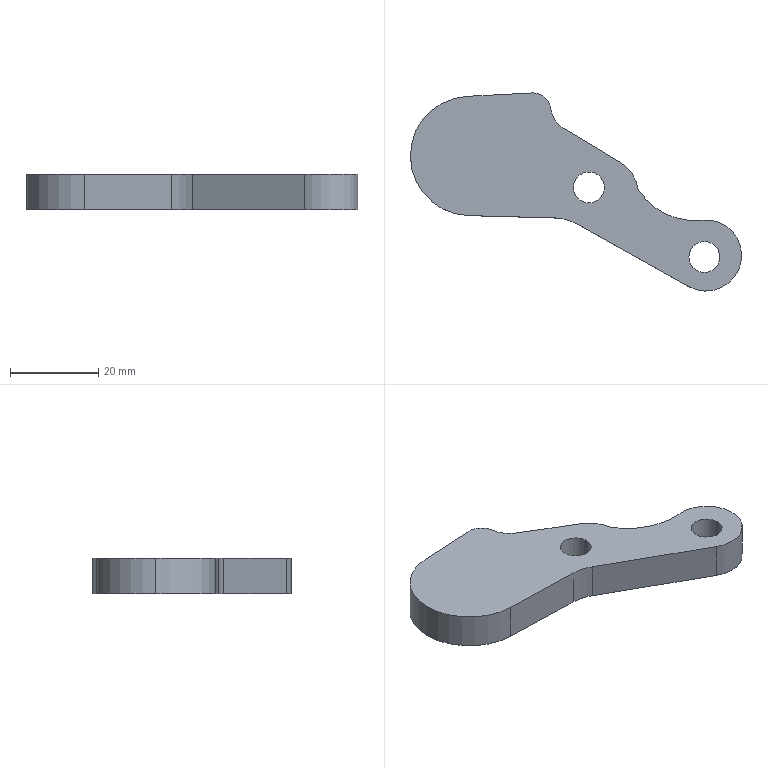Part | SolidWorks | features Extrusion 1 | 1 solid | 18 faces | box 74.927 x 44.837 x 8 mm | volume 11417 mm3 | cylinder 12 | plane 6 | commonest cylinder face diameters 7 x4 27 x2 8 x1 12 x1 16.097 x1 17 x1
STEP:
#1=CARTESIAN_POINT('',(22.619,-15.75,8.));
#2=VERTEX_POINT('',#1);
#3=CARTESIAN_POINT('',(29.619,-15.75,8.));
#4=VERTEX_POINT('',#3);
#5=CARTESIAN_POINT('',(26.119,-15.75,8.));
#6=DIRECTION('',(0.,0.,1.));
#7=DIRECTION('',(1.,0.,0.));
#8=AXIS2_PLACEMENT_3D('',#5,#6,#7);
#9=CIRCLE('',#8,3.5);
#10=EDGE_CURVE('',#2,#4,#9,.T.);
#11=ORIENTED_EDGE('',*,*,#10,.T.);
#12=CARTESIAN_POINT('',(29.619,-15.75,0.));
#13=VERTEX_POINT('',#12);
#14=CARTESIAN_POINT('',(29.619,-15.75,8.));
#15=DIRECTION('',(0.,0.,-1.));
#16=VECTOR('',#15,1000.);
#17=LINE('',#14,#16);
#18=EDGE_CURVE('',#4,#13,#17,.T.);
#19=ORIENTED_EDGE('',*,*,#18,.T.);
#20=CARTESIAN_POINT('',(22.619,-15.75,0.));
#21=VERTEX_POINT('',#20);
#22=CARTESIAN_POINT('',(26.119,-15.75,0.));
#23=DIRECTION('',(0.,0.,1.));
#24=DIRECTION('',(1.,0.,0.));
#25=AXIS2_PLACEMENT_3D('',#22,#23,#24);
#26=CIRCLE('',#25,3.5);
#27=EDGE_CURVE('',#21,#13,#26,.T.);
#28=ORIENTED_EDGE('',*,*,#27,.F.);
#29=CARTESIAN_POINT('',(22.619,-15.75,8.));
#30=DIRECTION('',(0.,0.,-1.));
#31=VECTOR('',#30,1000.);
#32=LINE('',#29,#31);
#33=EDGE_CURVE('',#2,#21,#32,.T.);
#34=ORIENTED_EDGE('',*,*,#33,.F.);
#35=EDGE_LOOP('',(#11,#19,#28,#34));
#36=FACE_OUTER_BOUND('',#35,.T.);
#37=CARTESIAN_POINT('',(26.119,-15.75,8.));
#38=DIRECTION('',(0.,0.,-1.));
#39=DIRECTION('',(-1.,0.,0.));
#40=AXIS2_PLACEMENT_3D('',#37,#38,#39);
#41=CYLINDRICAL_SURFACE('',#40,3.5);
#42=ADVANCED_FACE('',(#36),#41,.F.);
#43=CARTESIAN_POINT('',(-3.5,0.,8.));
#44=VERTEX_POINT('',#43);
#45=CARTESIAN_POINT('',(3.5,0.,8.));
#46=VERTEX_POINT('',#45);
#47=CARTESIAN_POINT('',(0.,0.,8.));
#48=DIRECTION('',(0.,0.,1.));
#49=DIRECTION('',(1.,0.,0.));
#50=AXIS2_PLACEMENT_3D('',#47,#48,#49);
#51=CIRCLE('',#50,3.5);
#52=EDGE_CURVE('',#44,#46,#51,.T.);
#53=ORIENTED_EDGE('',*,*,#52,.T.);
#54=CARTESIAN_POINT('',(3.5,0.,0.));
#55=VERTEX_POINT('',#54);
#56=CARTESIAN_POINT('',(3.5,0.,8.));
#57=DIRECTION('',(0.,0.,-1.));
#58=VECTOR('',#57,1000.);
#59=LINE('',#56,#58);
#60=EDGE_CURVE('',#46,#55,#59,.T.);
#61=ORIENTED_EDGE('',*,*,#60,.T.);
#62=CARTESIAN_POINT('',(-3.5,0.,0.));
#63=VERTEX_POINT('',#62);
#64=CARTESIAN_POINT('',(0.,0.,0.));
#65=DIRECTION('',(0.,0.,1.));
#66=DIRECTION('',(1.,0.,0.));
#67=AXIS2_PLACEMENT_3D('',#64,#65,#66);
#68=CIRCLE('',#67,3.5);
#69=EDGE_CURVE('',#63,#55,#68,.T.);
#70=ORIENTED_EDGE('',*,*,#69,.F.);
#71=CARTESIAN_POINT('',(-3.5,0.,8.));
#72=DIRECTION('',(0.,0.,-1.));
#73=VECTOR('',#72,1000.);
#74=LINE('',#71,#73);
#75=EDGE_CURVE('',#44,#63,#74,.T.);
#76=ORIENTED_EDGE('',*,*,#75,.F.);
#77=EDGE_LOOP('',(#53,#61,#70,#76));
#78=FACE_OUTER_BOUND('',#77,.T.);
#79=CARTESIAN_POINT('',(0.,0.,8.));
#80=DIRECTION('',(0.,0.,-1.));
#81=DIRECTION('',(-1.,0.,0.));
#82=AXIS2_PLACEMENT_3D('',#79,#80,#81);
#83=CYLINDRICAL_SURFACE('',#82,3.5);
#84=ADVANCED_FACE('',(#78),#83,.F.);
#85=CARTESIAN_POINT('',(-40.39,7.11,8.));
#86=VERTEX_POINT('',#85);
#87=CARTESIAN_POINT('',(-27.258,-6.385,8.));
#88=VERTEX_POINT('',#87);
#89=CARTESIAN_POINT('',(-26.89,7.11,8.));
#90=DIRECTION('',(0.,0.,1.));
#91=DIRECTION('',(1.,0.,0.));
#92=AXIS2_PLACEMENT_3D('',#89,#90,#91);
#93=CIRCLE('',#92,13.5);
#94=EDGE_CURVE('',#86,#88,#93,.T.);
#95=ORIENTED_EDGE('',*,*,#94,.F.);
#96=CARTESIAN_POINT('',(-40.39,7.11,0.));
#97=VERTEX_POINT('',#96);
#98=CARTESIAN_POINT('',(-40.39,7.11,8.));
#99=DIRECTION('',(0.,0.,-1.));
#100=VECTOR('',#99,1000.);
#101=LINE('',#98,#100);
#102=EDGE_CURVE('',#86,#97,#101,.T.);
#103=ORIENTED_EDGE('',*,*,#102,.T.);
#104=CARTESIAN_POINT('',(-27.258,-6.385,0.));
#105=VERTEX_POINT('',#104);
#106=CARTESIAN_POINT('',(-26.89,7.11,0.));
#107=DIRECTION('',(0.,0.,1.));
#108=DIRECTION('',(1.,0.,0.));
#109=AXIS2_PLACEMENT_3D('',#106,#107,#108);
#110=CIRCLE('',#109,13.5);
#111=EDGE_CURVE('',#97,#105,#110,.T.);
#112=ORIENTED_EDGE('',*,*,#111,.T.);
#113=CARTESIAN_POINT('',(-27.258,-6.385,8.));
#114=DIRECTION('',(0.,0.,-1.));
#115=VECTOR('',#114,1000.);
#116=LINE('',#113,#115);
#117=EDGE_CURVE('',#88,#105,#116,.T.);
#118=ORIENTED_EDGE('',*,*,#117,.F.);
#119=EDGE_LOOP('',(#95,#103,#112,#118));
#120=FACE_OUTER_BOUND('',#119,.T.);
#121=CARTESIAN_POINT('',(-26.89,7.11,8.));
#122=DIRECTION('',(0.,0.,-1.));
#123=DIRECTION('',(-1.,0.,0.));
#124=AXIS2_PLACEMENT_3D('',#121,#122,#123);
#125=CYLINDRICAL_SURFACE('',#124,13.5);
#126=ADVANCED_FACE('',(#120),#125,.T.);
#127=ORIENTED_EDGE('',*,*,#52,.F.);
#128=CARTESIAN_POINT('',(0.,0.,8.));
#129=DIRECTION('',(0.,0.,1.));
#130=DIRECTION('',(1.,0.,0.));
#131=AXIS2_PLACEMENT_3D('',#128,#129,#130);
#132=CIRCLE('',#131,3.5);
#133=EDGE_CURVE('',#46,#44,#132,.T.);
#134=ORIENTED_EDGE('',*,*,#133,.F.);
#135=EDGE_LOOP('',(#127,#134));
#136=FACE_BOUND('',#135,.T.);
#137=CARTESIAN_POINT('',(11.132,-0.4181,8.));
#138=VERTEX_POINT('',#137);
#139=CARTESIAN_POINT('',(7.109,5.639,8.));
#140=VERTEX_POINT('',#139);
#141=CARTESIAN_POINT('',(2.72,-1.64,8.));
#142=DIRECTION('',(0.,0.,1.));
#143=DIRECTION('',(1.,0.,0.));
#144=AXIS2_PLACEMENT_3D('',#141,#142,#143);
#145=CIRCLE('',#144,8.5);
#146=EDGE_CURVE('',#138,#140,#145,.T.);
#147=ORIENTED_EDGE('',*,*,#146,.T.);
#148=CARTESIAN_POINT('',(-5.798,13.422,8.));
#149=VERTEX_POINT('',#148);
#150=CARTESIAN_POINT('',(-5.798,13.422,8.));
#151=DIRECTION('',(-0.8564,0.5164,0.));
#152=VECTOR('',#151,1000.);
#153=LINE('',#150,#152);
#154=EDGE_CURVE('',#140,#149,#153,.T.);
#155=ORIENTED_EDGE('',*,*,#154,.T.);
#156=CARTESIAN_POINT('',(-8.658,17.851,8.));
#157=VERTEX_POINT('',#156);
#158=CARTESIAN_POINT('',(-2.7,18.56,8.));
#159=DIRECTION('',(0.,0.,-1.));
#160=DIRECTION('',(1.,0.,0.));
#161=AXIS2_PLACEMENT_3D('',#158,#159,#160);
#162=CIRCLE('',#161,6.);
#163=EDGE_CURVE('',#149,#157,#162,.T.);
#164=ORIENTED_EDGE('',*,*,#163,.T.);
#165=CARTESIAN_POINT('',(-12.842,21.373,8.));
#166=VERTEX_POINT('',#165);
#167=CARTESIAN_POINT('',(-12.63,17.379,8.));
#168=DIRECTION('',(0.,0.,1.));
#169=DIRECTION('',(1.,0.,0.));
#170=AXIS2_PLACEMENT_3D('',#167,#168,#169);
#171=CIRCLE('',#170,4.);
#172=EDGE_CURVE('',#157,#166,#171,.T.);
#173=ORIENTED_EDGE('',*,*,#172,.T.);
#174=CARTESIAN_POINT('',(-27.604,20.591,8.));
#175=VERTEX_POINT('',#174);
#176=CARTESIAN_POINT('',(-27.604,20.591,8.));
#177=DIRECTION('',(-0.9986,-0.05291,0.));
#178=VECTOR('',#177,1000.);
#179=LINE('',#176,#178);
#180=EDGE_CURVE('',#166,#175,#179,.T.);
#181=ORIENTED_EDGE('',*,*,#180,.T.);
#182=CARTESIAN_POINT('',(-26.89,7.11,8.));
#183=DIRECTION('',(0.,0.,1.));
#184=DIRECTION('',(1.,0.,0.));
#185=AXIS2_PLACEMENT_3D('',#182,#183,#184);
#186=CIRCLE('',#185,13.5);
#187=EDGE_CURVE('',#175,#86,#186,.T.);
#188=ORIENTED_EDGE('',*,*,#187,.T.);
#189=ORIENTED_EDGE('',*,*,#94,.T.);
#190=CARTESIAN_POINT('',(-7.488,-6.924,8.));
#191=VERTEX_POINT('',#190);
#192=CARTESIAN_POINT('',(-27.258,-6.385,8.));
#193=DIRECTION('',(0.9996,-0.02724,0.));
#194=VECTOR('',#193,1000.);
#195=LINE('',#192,#194);
#196=EDGE_CURVE('',#88,#191,#195,.T.);
#197=ORIENTED_EDGE('',*,*,#196,.T.);
#198=CARTESIAN_POINT('',(-2.875,-8.194,8.));
#199=VERTEX_POINT('',#198);
#200=CARTESIAN_POINT('',(-7.76,-16.92,8.));
#201=DIRECTION('',(0.,0.,-1.));
#202=DIRECTION('',(1.,0.,0.));
#203=AXIS2_PLACEMENT_3D('',#200,#201,#202);
#204=CIRCLE('',#203,10.);
#205=EDGE_CURVE('',#191,#199,#204,.T.);
#206=ORIENTED_EDGE('',*,*,#205,.T.);
#207=CARTESIAN_POINT('',(22.557,-22.432,8.));
#208=VERTEX_POINT('',#207);
#209=CARTESIAN_POINT('',(-2.875,-8.194,8.));
#210=DIRECTION('',(0.8726,-0.4885,0.));
#211=VECTOR('',#210,1000.);
#212=LINE('',#209,#211);
#213=EDGE_CURVE('',#199,#208,#212,.T.);
#214=ORIENTED_EDGE('',*,*,#213,.T.);
#215=CARTESIAN_POINT('',(25.577,-7.413,8.));
#216=VERTEX_POINT('',#215);
#217=CARTESIAN_POINT('',(26.489,-15.41,8.));
#218=DIRECTION('',(0.,0.,1.));
#219=DIRECTION('',(1.,0.,0.));
#220=AXIS2_PLACEMENT_3D('',#217,#218,#219);
#221=CIRCLE('',#220,8.048);
#222=EDGE_CURVE('',#208,#216,#221,.T.);
#223=ORIENTED_EDGE('',*,*,#222,.T.);
#224=CARTESIAN_POINT('',(23.878,7.49,8.));
#225=DIRECTION('',(0.,0.,-1.));
#226=DIRECTION('',(1.,0.,0.));
#227=AXIS2_PLACEMENT_3D('',#224,#225,#226);
#228=CIRCLE('',#227,15.);
#229=EDGE_CURVE('',#216,#138,#228,.T.);
#230=ORIENTED_EDGE('',*,*,#229,.T.);
#231=EDGE_LOOP('',(#147,#155,#164,#173,#181,#188,#189,#197,#206,#214,#223,#230));
#232=FACE_OUTER_BOUND('',#231,.T.);
#233=ORIENTED_EDGE('',*,*,#10,.F.);
#234=CARTESIAN_POINT('',(26.119,-15.75,8.));
#235=DIRECTION('',(0.,0.,1.));
#236=DIRECTION('',(1.,0.,0.));
#237=AXIS2_PLACEMENT_3D('',#234,#235,#236);
#238=CIRCLE('',#237,3.5);
#239=EDGE_CURVE('',#4,#2,#238,.T.);
#240=ORIENTED_EDGE('',*,*,#239,.F.);
#241=EDGE_LOOP('',(#233,#240));
#242=FACE_BOUND('',#241,.T.);
#243=CARTESIAN_POINT('',(2.72,-1.64,8.));
#244=DIRECTION('',(0.,0.,1.));
#245=DIRECTION('',(1.,0.,0.));
#246=AXIS2_PLACEMENT_3D('',#243,#244,#245);
#247=PLANE('',#246);
#248=ADVANCED_FACE('',(#136,#232,#242),#247,.T.);
#249=CARTESIAN_POINT('',(11.132,-0.4181,0.));
#250=VERTEX_POINT('',#249);
#251=CARTESIAN_POINT('',(7.109,5.639,0.));
#252=VERTEX_POINT('',#251);
#253=CARTESIAN_POINT('',(2.72,-1.64,0.));
#254=DIRECTION('',(0.,0.,1.));
#255=DIRECTION('',(1.,0.,0.));
#256=AXIS2_PLACEMENT_3D('',#253,#254,#255);
#257=CIRCLE('',#256,8.5);
#258=EDGE_CURVE('',#250,#252,#257,.T.);
#259=ORIENTED_EDGE('',*,*,#258,.F.);
#260=CARTESIAN_POINT('',(25.577,-7.413,0.));
#261=VERTEX_POINT('',#260);
#262=CARTESIAN_POINT('',(23.878,7.49,0.));
#263=DIRECTION('',(0.,0.,-1.));
#264=DIRECTION('',(1.,0.,0.));
#265=AXIS2_PLACEMENT_3D('',#262,#263,#264);
#266=CIRCLE('',#265,15.);
#267=EDGE_CURVE('',#261,#250,#266,.T.);
#268=ORIENTED_EDGE('',*,*,#267,.F.);
#269=CARTESIAN_POINT('',(22.557,-22.432,0.));
#270=VERTEX_POINT('',#269);
#271=CARTESIAN_POINT('',(26.489,-15.41,0.));
#272=DIRECTION('',(0.,0.,1.));
#273=DIRECTION('',(1.,0.,0.));
#274=AXIS2_PLACEMENT_3D('',#271,#272,#273);
#275=CIRCLE('',#274,8.048);
#276=EDGE_CURVE('',#270,#261,#275,.T.);
#277=ORIENTED_EDGE('',*,*,#276,.F.);
#278=CARTESIAN_POINT('',(-2.875,-8.194,0.));
#279=VERTEX_POINT('',#278);
#280=CARTESIAN_POINT('',(-2.875,-8.194,0.));
#281=DIRECTION('',(0.8726,-0.4885,0.));
#282=VECTOR('',#281,1000.);
#283=LINE('',#280,#282);
#284=EDGE_CURVE('',#279,#270,#283,.T.);
#285=ORIENTED_EDGE('',*,*,#284,.F.);
#286=CARTESIAN_POINT('',(-7.488,-6.924,0.));
#287=VERTEX_POINT('',#286);
#288=CARTESIAN_POINT('',(-7.76,-16.92,0.));
#289=DIRECTION('',(0.,0.,-1.));
#290=DIRECTION('',(1.,0.,0.));
#291=AXIS2_PLACEMENT_3D('',#288,#289,#290);
#292=CIRCLE('',#291,10.);
#293=EDGE_CURVE('',#287,#279,#292,.T.);
#294=ORIENTED_EDGE('',*,*,#293,.F.);
#295=CARTESIAN_POINT('',(-27.258,-6.385,0.));
#296=DIRECTION('',(0.9996,-0.02724,0.));
#297=VECTOR('',#296,1000.);
#298=LINE('',#295,#297);
#299=EDGE_CURVE('',#105,#287,#298,.T.);
#300=ORIENTED_EDGE('',*,*,#299,.F.);
#301=ORIENTED_EDGE('',*,*,#111,.F.);
#302=CARTESIAN_POINT('',(-27.604,20.591,0.));
#303=VERTEX_POINT('',#302);
#304=CARTESIAN_POINT('',(-26.89,7.11,0.));
#305=DIRECTION('',(0.,0.,1.));
#306=DIRECTION('',(1.,0.,0.));
#307=AXIS2_PLACEMENT_3D('',#304,#305,#306);
#308=CIRCLE('',#307,13.5);
#309=EDGE_CURVE('',#303,#97,#308,.T.);
#310=ORIENTED_EDGE('',*,*,#309,.F.);
#311=CARTESIAN_POINT('',(-12.842,21.373,0.));
#312=VERTEX_POINT('',#311);
#313=CARTESIAN_POINT('',(-27.604,20.591,0.));
#314=DIRECTION('',(-0.9986,-0.05291,0.));
#315=VECTOR('',#314,1000.);
#316=LINE('',#313,#315);
#317=EDGE_CURVE('',#312,#303,#316,.T.);
#318=ORIENTED_EDGE('',*,*,#317,.F.);
#319=CARTESIAN_POINT('',(-8.658,17.851,0.));
#320=VERTEX_POINT('',#319);
#321=CARTESIAN_POINT('',(-12.63,17.379,0.));
#322=DIRECTION('',(0.,0.,1.));
#323=DIRECTION('',(1.,0.,0.));
#324=AXIS2_PLACEMENT_3D('',#321,#322,#323);
#325=CIRCLE('',#324,4.);
#326=EDGE_CURVE('',#320,#312,#325,.T.);
#327=ORIENTED_EDGE('',*,*,#326,.F.);
#328=CARTESIAN_POINT('',(-5.798,13.422,0.));
#329=VERTEX_POINT('',#328);
#330=CARTESIAN_POINT('',(-2.7,18.56,0.));
#331=DIRECTION('',(0.,0.,-1.));
#332=DIRECTION('',(1.,0.,0.));
#333=AXIS2_PLACEMENT_3D('',#330,#331,#332);
#334=CIRCLE('',#333,6.);
#335=EDGE_CURVE('',#329,#320,#334,.T.);
#336=ORIENTED_EDGE('',*,*,#335,.F.);
#337=CARTESIAN_POINT('',(-5.798,13.422,0.));
#338=DIRECTION('',(-0.8564,0.5164,0.));
#339=VECTOR('',#338,1000.);
#340=LINE('',#337,#339);
#341=EDGE_CURVE('',#252,#329,#340,.T.);
#342=ORIENTED_EDGE('',*,*,#341,.F.);
#343=EDGE_LOOP('',(#259,#268,#277,#285,#294,#300,#301,#310,#318,#327,#336,#342));
#344=FACE_OUTER_BOUND('',#343,.T.);
#345=ORIENTED_EDGE('',*,*,#69,.T.);
#346=CARTESIAN_POINT('',(0.,0.,0.));
#347=DIRECTION('',(0.,0.,1.));
#348=DIRECTION('',(1.,0.,0.));
#349=AXIS2_PLACEMENT_3D('',#346,#347,#348);
#350=CIRCLE('',#349,3.5);
#351=EDGE_CURVE('',#55,#63,#350,.T.);
#352=ORIENTED_EDGE('',*,*,#351,.T.);
#353=EDGE_LOOP('',(#345,#352));
#354=FACE_BOUND('',#353,.T.);
#355=ORIENTED_EDGE('',*,*,#27,.T.);
#356=CARTESIAN_POINT('',(26.119,-15.75,0.));
#357=DIRECTION('',(0.,0.,1.));
#358=DIRECTION('',(1.,0.,0.));
#359=AXIS2_PLACEMENT_3D('',#356,#357,#358);
#360=CIRCLE('',#359,3.5);
#361=EDGE_CURVE('',#13,#21,#360,.T.);
#362=ORIENTED_EDGE('',*,*,#361,.T.);
#363=EDGE_LOOP('',(#355,#362));
#364=FACE_BOUND('',#363,.T.);
#365=CARTESIAN_POINT('',(2.72,-1.64,0.));
#366=DIRECTION('',(0.,0.,1.));
#367=DIRECTION('',(1.,0.,0.));
#368=AXIS2_PLACEMENT_3D('',#365,#366,#367);
#369=PLANE('',#368);
#370=ADVANCED_FACE('',(#344,#354,#364),#369,.F.);
#371=ORIENTED_EDGE('',*,*,#258,.T.);
#372=CARTESIAN_POINT('',(7.109,5.639,8.));
#373=DIRECTION('',(0.,0.,-1.));
#374=VECTOR('',#373,1000.);
#375=LINE('',#372,#374);
#376=EDGE_CURVE('',#140,#252,#375,.T.);
#377=ORIENTED_EDGE('',*,*,#376,.F.);
#378=ORIENTED_EDGE('',*,*,#146,.F.);
#379=CARTESIAN_POINT('',(11.132,-0.4181,8.));
#380=DIRECTION('',(0.,0.,-1.));
#381=VECTOR('',#380,1000.);
#382=LINE('',#379,#381);
#383=EDGE_CURVE('',#138,#250,#382,.T.);
#384=ORIENTED_EDGE('',*,*,#383,.T.);
#385=EDGE_LOOP('',(#371,#377,#378,#384));
#386=FACE_OUTER_BOUND('',#385,.T.);
#387=CARTESIAN_POINT('',(2.72,-1.64,8.));
#388=DIRECTION('',(0.,0.,-1.));
#389=DIRECTION('',(-1.,0.,0.));
#390=AXIS2_PLACEMENT_3D('',#387,#388,#389);
#391=CYLINDRICAL_SURFACE('',#390,8.5);
#392=ADVANCED_FACE('',(#386),#391,.T.);
#393=ORIENTED_EDGE('',*,*,#341,.T.);
#394=CARTESIAN_POINT('',(-5.798,13.422,8.));
#395=DIRECTION('',(0.,0.,-1.));
#396=VECTOR('',#395,1000.);
#397=LINE('',#394,#396);
#398=EDGE_CURVE('',#149,#329,#397,.T.);
#399=ORIENTED_EDGE('',*,*,#398,.F.);
#400=ORIENTED_EDGE('',*,*,#154,.F.);
#401=ORIENTED_EDGE('',*,*,#376,.T.);
#402=EDGE_LOOP('',(#393,#399,#400,#401));
#403=FACE_OUTER_BOUND('',#402,.T.);
#404=CARTESIAN_POINT('',(-5.798,13.422,8.));
#405=DIRECTION('',(-0.5164,-0.8564,0.));
#406=DIRECTION('',(0.8564,-0.5164,0.));
#407=AXIS2_PLACEMENT_3D('',#404,#405,#406);
#408=PLANE('',#407);
#409=ADVANCED_FACE('',(#403),#408,.F.);
#410=ORIENTED_EDGE('',*,*,#335,.T.);
#411=CARTESIAN_POINT('',(-8.658,17.851,8.));
#412=DIRECTION('',(0.,0.,-1.));
#413=VECTOR('',#412,1000.);
#414=LINE('',#411,#413);
#415=EDGE_CURVE('',#157,#320,#414,.T.);
#416=ORIENTED_EDGE('',*,*,#415,.F.);
#417=ORIENTED_EDGE('',*,*,#163,.F.);
#418=ORIENTED_EDGE('',*,*,#398,.T.);
#419=EDGE_LOOP('',(#410,#416,#417,#418));
#420=FACE_OUTER_BOUND('',#419,.T.);
#421=CARTESIAN_POINT('',(-2.7,18.56,8.));
#422=DIRECTION('',(0.,0.,-1.));
#423=DIRECTION('',(-1.,0.,0.));
#424=AXIS2_PLACEMENT_3D('',#421,#422,#423);
#425=CYLINDRICAL_SURFACE('',#424,6.);
#426=ADVANCED_FACE('',(#420),#425,.F.);
#427=ORIENTED_EDGE('',*,*,#326,.T.);
#428=CARTESIAN_POINT('',(-12.842,21.373,8.));
#429=DIRECTION('',(0.,0.,-1.));
#430=VECTOR('',#429,1000.);
#431=LINE('',#428,#430);
#432=EDGE_CURVE('',#166,#312,#431,.T.);
#433=ORIENTED_EDGE('',*,*,#432,.F.);
#434=ORIENTED_EDGE('',*,*,#172,.F.);
#435=ORIENTED_EDGE('',*,*,#415,.T.);
#436=EDGE_LOOP('',(#427,#433,#434,#435));
#437=FACE_OUTER_BOUND('',#436,.T.);
#438=CARTESIAN_POINT('',(-12.63,17.379,8.));
#439=DIRECTION('',(0.,0.,-1.));
#440=DIRECTION('',(-1.,0.,0.));
#441=AXIS2_PLACEMENT_3D('',#438,#439,#440);
#442=CYLINDRICAL_SURFACE('',#441,4.);
#443=ADVANCED_FACE('',(#437),#442,.T.);
#444=ORIENTED_EDGE('',*,*,#317,.T.);
#445=CARTESIAN_POINT('',(-27.604,20.591,8.));
#446=DIRECTION('',(0.,0.,-1.));
#447=VECTOR('',#446,1000.);
#448=LINE('',#445,#447);
#449=EDGE_CURVE('',#175,#303,#448,.T.);
#450=ORIENTED_EDGE('',*,*,#449,.F.);
#451=ORIENTED_EDGE('',*,*,#180,.F.);
#452=ORIENTED_EDGE('',*,*,#432,.T.);
#453=EDGE_LOOP('',(#444,#450,#451,#452));
#454=FACE_OUTER_BOUND('',#453,.T.);
#455=CARTESIAN_POINT('',(-27.604,20.591,8.));
#456=DIRECTION('',(0.05291,-0.9986,0.));
#457=DIRECTION('',(0.9986,0.05291,0.));
#458=AXIS2_PLACEMENT_3D('',#455,#456,#457);
#459=PLANE('',#458);
#460=ADVANCED_FACE('',(#454),#459,.F.);
#461=ORIENTED_EDGE('',*,*,#102,.F.);
#462=ORIENTED_EDGE('',*,*,#187,.F.);
#463=ORIENTED_EDGE('',*,*,#449,.T.);
#464=ORIENTED_EDGE('',*,*,#309,.T.);
#465=EDGE_LOOP('',(#461,#462,#463,#464));
#466=FACE_OUTER_BOUND('',#465,.T.);
#467=CARTESIAN_POINT('',(-26.89,7.11,8.));
#468=DIRECTION('',(0.,0.,-1.));
#469=DIRECTION('',(-1.,0.,0.));
#470=AXIS2_PLACEMENT_3D('',#467,#468,#469);
#471=CYLINDRICAL_SURFACE('',#470,13.5);
#472=ADVANCED_FACE('',(#466),#471,.T.);
#473=ORIENTED_EDGE('',*,*,#299,.T.);
#474=CARTESIAN_POINT('',(-7.488,-6.924,8.));
#475=DIRECTION('',(0.,0.,-1.));
#476=VECTOR('',#475,1000.);
#477=LINE('',#474,#476);
#478=EDGE_CURVE('',#191,#287,#477,.T.);
#479=ORIENTED_EDGE('',*,*,#478,.F.);
#480=ORIENTED_EDGE('',*,*,#196,.F.);
#481=ORIENTED_EDGE('',*,*,#117,.T.);
#482=EDGE_LOOP('',(#473,#479,#480,#481));
#483=FACE_OUTER_BOUND('',#482,.T.);
#484=CARTESIAN_POINT('',(-27.258,-6.385,8.));
#485=DIRECTION('',(0.02724,0.9996,0.));
#486=DIRECTION('',(-0.9996,0.02724,0.));
#487=AXIS2_PLACEMENT_3D('',#484,#485,#486);
#488=PLANE('',#487);
#489=ADVANCED_FACE('',(#483),#488,.F.);
#490=ORIENTED_EDGE('',*,*,#293,.T.);
#491=CARTESIAN_POINT('',(-2.875,-8.194,8.));
#492=DIRECTION('',(0.,0.,-1.));
#493=VECTOR('',#492,1000.);
#494=LINE('',#491,#493);
#495=EDGE_CURVE('',#199,#279,#494,.T.);
#496=ORIENTED_EDGE('',*,*,#495,.F.);
#497=ORIENTED_EDGE('',*,*,#205,.F.);
#498=ORIENTED_EDGE('',*,*,#478,.T.);
#499=EDGE_LOOP('',(#490,#496,#497,#498));
#500=FACE_OUTER_BOUND('',#499,.T.);
#501=CARTESIAN_POINT('',(-7.76,-16.92,8.));
#502=DIRECTION('',(0.,0.,-1.));
#503=DIRECTION('',(-1.,0.,0.));
#504=AXIS2_PLACEMENT_3D('',#501,#502,#503);
#505=CYLINDRICAL_SURFACE('',#504,10.);
#506=ADVANCED_FACE('',(#500),#505,.F.);
#507=ORIENTED_EDGE('',*,*,#284,.T.);
#508=CARTESIAN_POINT('',(22.557,-22.432,8.));
#509=DIRECTION('',(0.,0.,-1.));
#510=VECTOR('',#509,1000.);
#511=LINE('',#508,#510);
#512=EDGE_CURVE('',#208,#270,#511,.T.);
#513=ORIENTED_EDGE('',*,*,#512,.F.);
#514=ORIENTED_EDGE('',*,*,#213,.F.);
#515=ORIENTED_EDGE('',*,*,#495,.T.);
#516=EDGE_LOOP('',(#507,#513,#514,#515));
#517=FACE_OUTER_BOUND('',#516,.T.);
#518=CARTESIAN_POINT('',(-2.875,-8.194,8.));
#519=DIRECTION('',(0.4885,0.8726,0.));
#520=DIRECTION('',(-0.8726,0.4885,0.));
#521=AXIS2_PLACEMENT_3D('',#518,#519,#520);
#522=PLANE('',#521);
#523=ADVANCED_FACE('',(#517),#522,.F.);
#524=ORIENTED_EDGE('',*,*,#276,.T.);
#525=CARTESIAN_POINT('',(25.577,-7.413,8.));
#526=DIRECTION('',(0.,0.,-1.));
#527=VECTOR('',#526,1000.);
#528=LINE('',#525,#527);
#529=EDGE_CURVE('',#216,#261,#528,.T.);
#530=ORIENTED_EDGE('',*,*,#529,.F.);
#531=ORIENTED_EDGE('',*,*,#222,.F.);
#532=ORIENTED_EDGE('',*,*,#512,.T.);
#533=EDGE_LOOP('',(#524,#530,#531,#532));
#534=FACE_OUTER_BOUND('',#533,.T.);
#535=CARTESIAN_POINT('',(26.489,-15.41,8.));
#536=DIRECTION('',(0.,0.,-1.));
#537=DIRECTION('',(-1.,0.,0.));
#538=AXIS2_PLACEMENT_3D('',#535,#536,#537);
#539=CYLINDRICAL_SURFACE('',#538,8.048);
#540=ADVANCED_FACE('',(#534),#539,.T.);
#541=ORIENTED_EDGE('',*,*,#267,.T.);
#542=ORIENTED_EDGE('',*,*,#383,.F.);
#543=ORIENTED_EDGE('',*,*,#229,.F.);
#544=ORIENTED_EDGE('',*,*,#529,.T.);
#545=EDGE_LOOP('',(#541,#542,#543,#544));
#546=FACE_OUTER_BOUND('',#545,.T.);
#547=CARTESIAN_POINT('',(23.878,7.49,8.));
#548=DIRECTION('',(0.,0.,-1.));
#549=DIRECTION('',(-1.,0.,0.));
#550=AXIS2_PLACEMENT_3D('',#547,#548,#549);
#551=CYLINDRICAL_SURFACE('',#550,15.);
#552=ADVANCED_FACE('',(#546),#551,.F.);
#553=ORIENTED_EDGE('',*,*,#60,.F.);
#554=ORIENTED_EDGE('',*,*,#133,.T.);
#555=ORIENTED_EDGE('',*,*,#75,.T.);
#556=ORIENTED_EDGE('',*,*,#351,.F.);
#557=EDGE_LOOP('',(#553,#554,#555,#556));
#558=FACE_OUTER_BOUND('',#557,.T.);
#559=CARTESIAN_POINT('',(0.,0.,8.));
#560=DIRECTION('',(0.,0.,-1.));
#561=DIRECTION('',(-1.,0.,0.));
#562=AXIS2_PLACEMENT_3D('',#559,#560,#561);
#563=CYLINDRICAL_SURFACE('',#562,3.5);
#564=ADVANCED_FACE('',(#558),#563,.F.);
#565=ORIENTED_EDGE('',*,*,#18,.F.);
#566=ORIENTED_EDGE('',*,*,#239,.T.);
#567=ORIENTED_EDGE('',*,*,#33,.T.);
#568=ORIENTED_EDGE('',*,*,#361,.F.);
#569=EDGE_LOOP('',(#565,#566,#567,#568));
#570=FACE_OUTER_BOUND('',#569,.T.);
#571=CARTESIAN_POINT('',(26.119,-15.75,8.));
#572=DIRECTION('',(0.,0.,-1.));
#573=DIRECTION('',(-1.,0.,0.));
#574=AXIS2_PLACEMENT_3D('',#571,#572,#573);
#575=CYLINDRICAL_SURFACE('',#574,3.5);
#576=ADVANCED_FACE('',(#570),#575,.F.);
#577=CLOSED_SHELL('',(#42,#84,#126,#248,#370,#392,#409,#426,#443,#460,#472,#489,#506,#523,#540,#552,#564,#576));
#578=MANIFOLD_SOLID_BREP('',#577);
#579=CARTESIAN_POINT('',(0.,0.,0.));
#580=DIRECTION('',(0.,0.,1.));
#581=DIRECTION('',(1.,0.,0.));
#582=AXIS2_PLACEMENT_3D('',#579,#580,#581);
#583=(LENGTH_UNIT()NAMED_UNIT(*)SI_UNIT(.MILLI.,.METRE.));
#584=UNCERTAINTY_MEASURE_WITH_UNIT(LENGTH_MEASURE(0.00001),#583,'','');
#585=(NAMED_UNIT(*)PLANE_ANGLE_UNIT()SI_UNIT($,.RADIAN.));
#586=(NAMED_UNIT(*)SI_UNIT($,.STERADIAN.)SOLID_ANGLE_UNIT());
#587=(GEOMETRIC_REPRESENTATION_CONTEXT(3)GLOBAL_UNCERTAINTY_ASSIGNED_CONTEXT((#584))GLOBAL_UNIT_ASSIGNED_CONTEXT((#583,#585,#586))REPRESENTATION_CONTEXT('',''));
#588=ADVANCED_BREP_SHAPE_REPRESENTATION('',(#578,#582),#587);